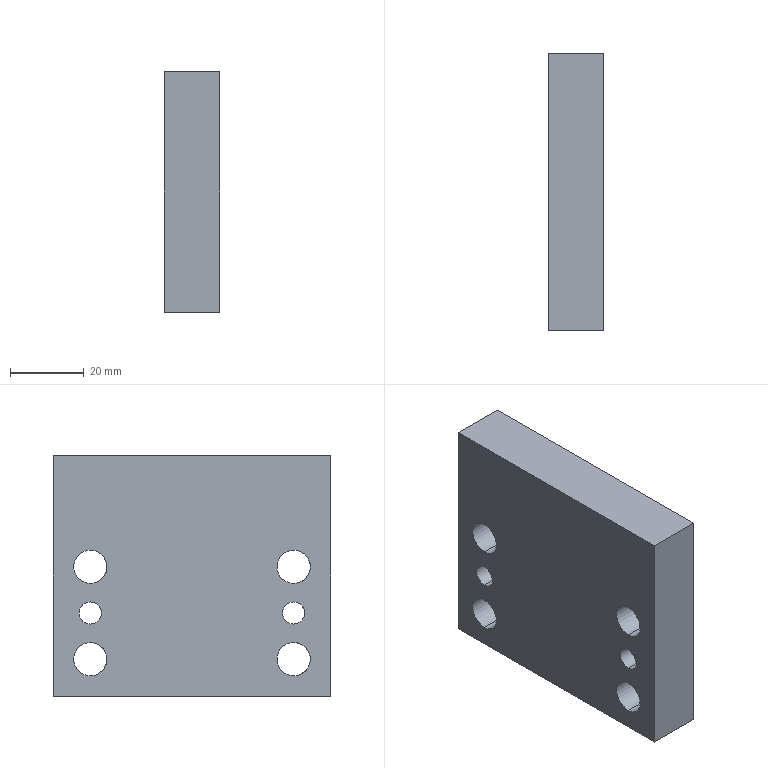Part | STEP file | Positioning_id1210_x_t | 1 solid | 18 faces | box 15 x 75 x 65 mm | volume 68460 mm3 | cylinder 12 | plane 6 | commonest cylinder face diameters 9 x8 6 x4